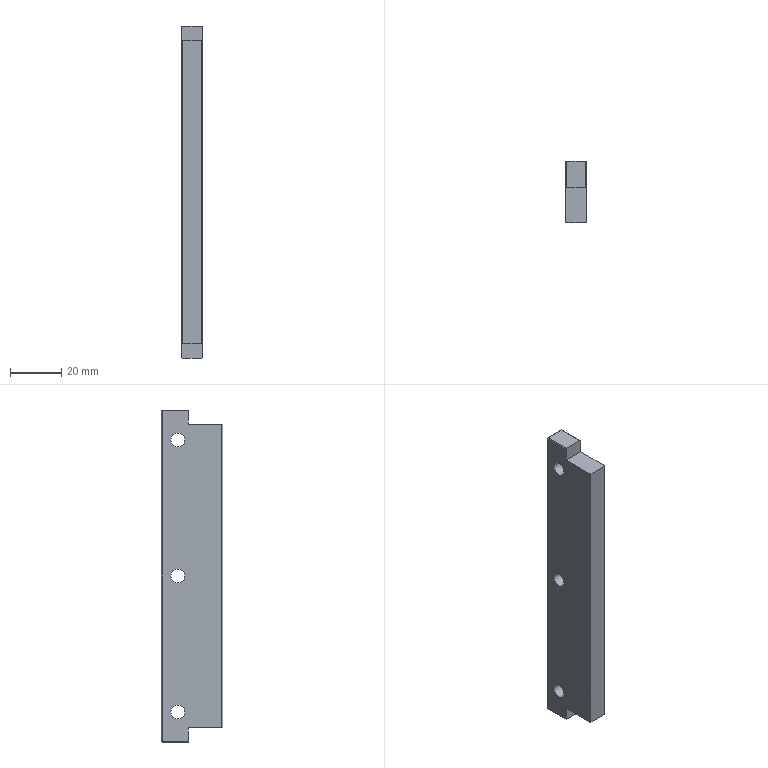Part | NX | 1 solid | 26 faces | box 8 x 24 x 130 mm | volume 23177 mm3 | plane 20 | cylinder 6 | commonest cylinder face diameters 5.5 x6
STEP:
#1=CARTESIAN_POINT('',(1727.3,110.5,87.2));
#2=VERTEX_POINT('',#1);
#3=CARTESIAN_POINT('',(1734.7,110.5,87.2));
#4=VERTEX_POINT('',#3);
#5=CARTESIAN_POINT('',(1731.,110.5,87.2));
#6=DIRECTION('',(1.,0.,0.));
#7=VECTOR('',#6,1000.);
#8=LINE('',#5,#7);
#9=EDGE_CURVE('',#2,#4,#8,.T.);
#10=ORIENTED_EDGE('',*,*,#9,.T.);
#11=CARTESIAN_POINT('',(1734.7,110.5,-42.2));
#12=VERTEX_POINT('',#11);
#13=CARTESIAN_POINT('',(1734.7,110.5,22.5));
#14=DIRECTION('',(0.,0.,1.));
#15=VECTOR('',#14,1000.);
#16=LINE('',#13,#15);
#17=EDGE_CURVE('',#12,#4,#16,.T.);
#18=ORIENTED_EDGE('',*,*,#17,.F.);
#19=CARTESIAN_POINT('',(1727.3,110.5,-42.2));
#20=VERTEX_POINT('',#19);
#21=CARTESIAN_POINT('',(1731.,110.5,-42.2));
#22=DIRECTION('',(-1.,0.,0.));
#23=VECTOR('',#22,1000.);
#24=LINE('',#21,#23);
#25=EDGE_CURVE('',#12,#20,#24,.T.);
#26=ORIENTED_EDGE('',*,*,#25,.T.);
#27=CARTESIAN_POINT('',(1727.3,110.5,22.5));
#28=DIRECTION('',(0.,0.,1.));
#29=VECTOR('',#28,1000.);
#30=LINE('',#27,#29);
#31=EDGE_CURVE('',#20,#2,#30,.T.);
#32=ORIENTED_EDGE('',*,*,#31,.T.);
#33=EDGE_LOOP('',(#10,#18,#26,#32));
#34=FACE_BOUND('',#33,.T.);
#35=CARTESIAN_POINT('',(1727.,110.5,93.5));
#36=DIRECTION('',(0.,1.,0.));
#37=DIRECTION('',(1.,0.,0.));
#38=AXIS2_PLACEMENT_3D('',#35,#36,#37);
#39=PLANE('',#38);
#40=ADVANCED_FACE('',(#34),#39,.T.);
#41=CARTESIAN_POINT('',(1734.7,100.,87.5));
#42=VERTEX_POINT('',#41);
#43=CARTESIAN_POINT('',(1727.3,100.,87.5));
#44=VERTEX_POINT('',#43);
#45=CARTESIAN_POINT('',(1727.,100.,87.5));
#46=DIRECTION('',(-1.,0.,0.));
#47=VECTOR('',#46,1000.);
#48=LINE('',#45,#47);
#49=EDGE_CURVE('',#42,#44,#48,.T.);
#50=ORIENTED_EDGE('',*,*,#49,.F.);
#51=CARTESIAN_POINT('',(1734.7,110.2,87.5));
#52=VERTEX_POINT('',#51);
#53=CARTESIAN_POINT('',(1734.7,103.803,87.5));
#54=DIRECTION('',(0.,-1.,0.));
#55=VECTOR('',#54,1000.);
#56=LINE('',#53,#55);
#57=EDGE_CURVE('',#52,#42,#56,.T.);
#58=ORIENTED_EDGE('',*,*,#57,.F.);
#59=CARTESIAN_POINT('',(1727.3,110.2,87.5));
#60=VERTEX_POINT('',#59);
#61=CARTESIAN_POINT('',(1731.,110.2,87.5));
#62=DIRECTION('',(1.,0.,0.));
#63=VECTOR('',#62,1000.);
#64=LINE('',#61,#63);
#65=EDGE_CURVE('',#60,#52,#64,.T.);
#66=ORIENTED_EDGE('',*,*,#65,.F.);
#67=CARTESIAN_POINT('',(1727.3,103.803,87.5));
#68=DIRECTION('',(0.,-1.,0.));
#69=VECTOR('',#68,1000.);
#70=LINE('',#67,#69);
#71=EDGE_CURVE('',#60,#44,#70,.T.);
#72=ORIENTED_EDGE('',*,*,#71,.T.);
#73=EDGE_LOOP('',(#50,#58,#66,#72));
#74=FACE_BOUND('',#73,.T.);
#75=CARTESIAN_POINT('',(1727.,88.5,87.5));
#76=DIRECTION('',(0.,0.,1.));
#77=DIRECTION('',(1.,0.,0.));
#78=AXIS2_PLACEMENT_3D('',#75,#76,#77);
#79=PLANE('',#78);
#80=ADVANCED_FACE('',(#74),#79,.T.);
#81=CARTESIAN_POINT('',(1727.,86.8,-37.));
#82=VERTEX_POINT('',#81);
#83=CARTESIAN_POINT('',(1727.,100.,-37.));
#84=VERTEX_POINT('',#83);
#85=CARTESIAN_POINT('',(1727.,0.,-37.));
#86=DIRECTION('',(0.,1.,0.));
#87=VECTOR('',#86,1000.);
#88=LINE('',#85,#87);
#89=EDGE_CURVE('',#82,#84,#88,.T.);
#90=ORIENTED_EDGE('',*,*,#89,.T.);
#91=CARTESIAN_POINT('',(1735.,100.,-37.));
#92=VERTEX_POINT('',#91);
#93=CARTESIAN_POINT('',(1727.,100.,-37.));
#94=DIRECTION('',(-1.,0.,0.));
#95=VECTOR('',#94,1000.);
#96=LINE('',#93,#95);
#97=EDGE_CURVE('',#92,#84,#96,.T.);
#98=ORIENTED_EDGE('',*,*,#97,.F.);
#99=CARTESIAN_POINT('',(1735.,86.8,-37.));
#100=VERTEX_POINT('',#99);
#101=CARTESIAN_POINT('',(1735.,103.803,-37.));
#102=DIRECTION('',(0.,-1.,0.));
#103=VECTOR('',#102,1000.);
#104=LINE('',#101,#103);
#105=EDGE_CURVE('',#92,#100,#104,.T.);
#106=ORIENTED_EDGE('',*,*,#105,.T.);
#107=CARTESIAN_POINT('',(1734.7,86.5,-37.));
#108=VERTEX_POINT('',#107);
#109=CARTESIAN_POINT('',(1752.003,103.803,-37.));
#110=DIRECTION('',(-0.7071,-0.7071,0.));
#111=VECTOR('',#110,1000.);
#112=LINE('',#109,#111);
#113=EDGE_CURVE('',#100,#108,#112,.T.);
#114=ORIENTED_EDGE('',*,*,#113,.T.);
#115=CARTESIAN_POINT('',(1727.3,86.5,-37.));
#116=VERTEX_POINT('',#115);
#117=CARTESIAN_POINT('',(1727.,86.5,-37.));
#118=DIRECTION('',(-1.,0.,0.));
#119=VECTOR('',#118,1000.);
#120=LINE('',#117,#119);
#121=EDGE_CURVE('',#108,#116,#120,.T.);
#122=ORIENTED_EDGE('',*,*,#121,.T.);
#123=CARTESIAN_POINT('',(1709.997,103.803,-37.));
#124=DIRECTION('',(0.7071,-0.7071,0.));
#125=VECTOR('',#124,1000.);
#126=LINE('',#123,#125);
#127=EDGE_CURVE('',#82,#116,#126,.T.);
#128=ORIENTED_EDGE('',*,*,#127,.F.);
#129=EDGE_LOOP('',(#90,#98,#106,#114,#122,#128));
#130=FACE_BOUND('',#129,.T.);
#131=CARTESIAN_POINT('',(1735.8,99.5,-37.));
#132=DIRECTION('',(0.,0.,1.));
#133=DIRECTION('',(1.,0.,0.));
#134=AXIS2_PLACEMENT_3D('',#131,#132,#133);
#135=PLANE('',#134);
#136=ADVANCED_FACE('',(#130),#135,.F.);
#137=CARTESIAN_POINT('',(1727.3,100.,-42.5));
#138=VERTEX_POINT('',#137);
#139=CARTESIAN_POINT('',(1727.3,110.2,-42.5));
#140=VERTEX_POINT('',#139);
#141=CARTESIAN_POINT('',(1727.3,103.803,-42.5));
#142=DIRECTION('',(0.,1.,0.));
#143=VECTOR('',#142,1000.);
#144=LINE('',#141,#143);
#145=EDGE_CURVE('',#138,#140,#144,.T.);
#146=ORIENTED_EDGE('',*,*,#145,.T.);
#147=CARTESIAN_POINT('',(1734.7,110.2,-42.5));
#148=VERTEX_POINT('',#147);
#149=CARTESIAN_POINT('',(1731.,110.2,-42.5));
#150=DIRECTION('',(-1.,0.,0.));
#151=VECTOR('',#150,1000.);
#152=LINE('',#149,#151);
#153=EDGE_CURVE('',#148,#140,#152,.T.);
#154=ORIENTED_EDGE('',*,*,#153,.F.);
#155=CARTESIAN_POINT('',(1734.7,100.,-42.5));
#156=VERTEX_POINT('',#155);
#157=CARTESIAN_POINT('',(1734.7,103.803,-42.5));
#158=DIRECTION('',(0.,1.,0.));
#159=VECTOR('',#158,1000.);
#160=LINE('',#157,#159);
#161=EDGE_CURVE('',#156,#148,#160,.T.);
#162=ORIENTED_EDGE('',*,*,#161,.F.);
#163=CARTESIAN_POINT('',(1727.,100.,-42.5));
#164=DIRECTION('',(1.,0.,0.));
#165=VECTOR('',#164,1000.);
#166=LINE('',#163,#165);
#167=EDGE_CURVE('',#138,#156,#166,.T.);
#168=ORIENTED_EDGE('',*,*,#167,.F.);
#169=EDGE_LOOP('',(#146,#154,#162,#168));
#170=FACE_BOUND('',#169,.T.);
#171=CARTESIAN_POINT('',(1727.,110.5,-42.5));
#172=DIRECTION('',(0.,0.,-1.));
#173=DIRECTION('',(0.,-1.,0.));
#174=AXIS2_PLACEMENT_3D('',#171,#172,#173);
#175=PLANE('',#174);
#176=ADVANCED_FACE('',(#170),#175,.T.);
#177=ORIENTED_EDGE('',*,*,#121,.F.);
#178=CARTESIAN_POINT('',(1734.7,86.5,82.));
#179=VERTEX_POINT('',#178);
#180=CARTESIAN_POINT('',(1734.7,86.5,-14.233));
#181=DIRECTION('',(0.,0.,-1.));
#182=VECTOR('',#181,1000.);
#183=LINE('',#180,#182);
#184=EDGE_CURVE('',#179,#108,#183,.T.);
#185=ORIENTED_EDGE('',*,*,#184,.F.);
#186=CARTESIAN_POINT('',(1727.3,86.5,82.));
#187=VERTEX_POINT('',#186);
#188=CARTESIAN_POINT('',(1727.,86.5,82.));
#189=DIRECTION('',(1.,0.,0.));
#190=VECTOR('',#189,1000.);
#191=LINE('',#188,#190);
#192=EDGE_CURVE('',#187,#179,#191,.T.);
#193=ORIENTED_EDGE('',*,*,#192,.F.);
#194=CARTESIAN_POINT('',(1727.3,86.5,-14.233));
#195=DIRECTION('',(0.,0.,-1.));
#196=VECTOR('',#195,1000.);
#197=LINE('',#194,#196);
#198=EDGE_CURVE('',#187,#116,#197,.T.);
#199=ORIENTED_EDGE('',*,*,#198,.T.);
#200=EDGE_LOOP('',(#177,#185,#193,#199));
#201=FACE_BOUND('',#200,.T.);
#202=CARTESIAN_POINT('',(1727.,86.5,-48.5));
#203=DIRECTION('',(0.,-1.,0.));
#204=DIRECTION('',(0.,0.,-1.));
#205=AXIS2_PLACEMENT_3D('',#202,#203,#204);
#206=PLANE('',#205);
#207=ADVANCED_FACE('',(#201),#206,.T.);
#208=ORIENTED_EDGE('',*,*,#25,.F.);
#209=CARTESIAN_POINT('',(1734.85,110.35,-42.35));
#210=VERTEX_POINT('',#209);
#211=CARTESIAN_POINT('',(1706.733,138.467,-14.233));
#212=DIRECTION('',(0.5774,-0.5774,-0.5774));
#213=VECTOR('',#212,1000.);
#214=LINE('',#211,#213);
#215=EDGE_CURVE('',#12,#210,#214,.T.);
#216=ORIENTED_EDGE('',*,*,#215,.T.);
#217=CARTESIAN_POINT('',(1762.967,138.467,-14.233));
#218=DIRECTION('',(0.5774,0.5774,0.5774));
#219=VECTOR('',#218,1000.);
#220=LINE('',#217,#219);
#221=EDGE_CURVE('',#148,#210,#220,.T.);
#222=ORIENTED_EDGE('',*,*,#221,.F.);
#223=ORIENTED_EDGE('',*,*,#153,.T.);
#224=CARTESIAN_POINT('',(1727.15,110.35,-42.35));
#225=VERTEX_POINT('',#224);
#226=CARTESIAN_POINT('',(1699.033,138.467,-14.233));
#227=DIRECTION('',(-0.5774,0.5774,0.5774));
#228=VECTOR('',#227,1000.);
#229=LINE('',#226,#228);
#230=EDGE_CURVE('',#140,#225,#229,.T.);
#231=ORIENTED_EDGE('',*,*,#230,.T.);
#232=CARTESIAN_POINT('',(1755.267,138.467,-14.233));
#233=DIRECTION('',(-0.5774,-0.5774,-0.5774));
#234=VECTOR('',#233,1000.);
#235=LINE('',#232,#234);
#236=EDGE_CURVE('',#20,#225,#235,.T.);
#237=ORIENTED_EDGE('',*,*,#236,.F.);
#238=EDGE_LOOP('',(#208,#216,#222,#223,#231,#237));
#239=FACE_BOUND('',#238,.T.);
#240=CARTESIAN_POINT('',(1731.,110.35,-42.35));
#241=DIRECTION('',(0.,0.7071,-0.7071));
#242=DIRECTION('',(-1.,0.,0.));
#243=AXIS2_PLACEMENT_3D('',#240,#241,#242);
#244=PLANE('',#243);
#245=ADVANCED_FACE('',(#239),#244,.T.);
#246=ORIENTED_EDGE('',*,*,#9,.F.);
#247=CARTESIAN_POINT('',(1727.15,110.35,87.35));
#248=VERTEX_POINT('',#247);
#249=CARTESIAN_POINT('',(1727.,110.2,87.5));
#250=DIRECTION('',(-0.5774,-0.5774,0.5774));
#251=VECTOR('',#250,1000.);
#252=LINE('',#249,#251);
#253=EDGE_CURVE('',#2,#248,#252,.T.);
#254=ORIENTED_EDGE('',*,*,#253,.T.);
#255=CARTESIAN_POINT('',(1733.697,103.803,93.897));
#256=DIRECTION('',(-0.5774,0.5774,-0.5774));
#257=VECTOR('',#256,1000.);
#258=LINE('',#255,#257);
#259=EDGE_CURVE('',#60,#248,#258,.T.);
#260=ORIENTED_EDGE('',*,*,#259,.F.);
#261=ORIENTED_EDGE('',*,*,#65,.T.);
#262=CARTESIAN_POINT('',(1734.85,110.35,87.35));
#263=VERTEX_POINT('',#262);
#264=CARTESIAN_POINT('',(1728.303,103.803,93.897));
#265=DIRECTION('',(0.5774,0.5774,-0.5774));
#266=VECTOR('',#265,1000.);
#267=LINE('',#264,#266);
#268=EDGE_CURVE('',#52,#263,#267,.T.);
#269=ORIENTED_EDGE('',*,*,#268,.T.);
#270=CARTESIAN_POINT('',(1741.397,103.803,93.897));
#271=DIRECTION('',(0.5774,-0.5774,0.5774));
#272=VECTOR('',#271,1000.);
#273=LINE('',#270,#272);
#274=EDGE_CURVE('',#4,#263,#273,.T.);
#275=ORIENTED_EDGE('',*,*,#274,.F.);
#276=EDGE_LOOP('',(#246,#254,#260,#261,#269,#275));
#277=FACE_BOUND('',#276,.T.);
#278=CARTESIAN_POINT('',(1731.,110.35,87.35));
#279=DIRECTION('',(0.,0.7071,0.7071));
#280=DIRECTION('',(1.,0.,0.));
#281=AXIS2_PLACEMENT_3D('',#278,#279,#280);
#282=PLANE('',#281);
#283=ADVANCED_FACE('',(#277),#282,.T.);
#284=CARTESIAN_POINT('',(1727.,100.,-42.2));
#285=VERTEX_POINT('',#284);
#286=CARTESIAN_POINT('',(1727.,100.,0.));
#287=DIRECTION('',(0.,0.,-1.));
#288=VECTOR('',#287,1000.);
#289=LINE('',#286,#288);
#290=EDGE_CURVE('',#84,#285,#289,.T.);
#291=ORIENTED_EDGE('',*,*,#290,.T.);
#292=CARTESIAN_POINT('',(1699.033,100.,-14.233));
#293=DIRECTION('',(-0.7071,0.,0.7071));
#294=VECTOR('',#293,1000.);
#295=LINE('',#292,#294);
#296=EDGE_CURVE('',#138,#285,#295,.T.);
#297=ORIENTED_EDGE('',*,*,#296,.F.);
#298=ORIENTED_EDGE('',*,*,#167,.T.);
#299=CARTESIAN_POINT('',(1735.,100.,-42.2));
#300=VERTEX_POINT('',#299);
#301=CARTESIAN_POINT('',(1762.967,100.,-14.233));
#302=DIRECTION('',(0.7071,0.,0.7071));
#303=VECTOR('',#302,1000.);
#304=LINE('',#301,#303);
#305=EDGE_CURVE('',#156,#300,#304,.T.);
#306=ORIENTED_EDGE('',*,*,#305,.T.);
#307=CARTESIAN_POINT('',(1735.,100.,-14.233));
#308=DIRECTION('',(0.,0.,1.));
#309=VECTOR('',#308,1000.);
#310=LINE('',#307,#309);
#311=EDGE_CURVE('',#300,#92,#310,.T.);
#312=ORIENTED_EDGE('',*,*,#311,.T.);
#313=ORIENTED_EDGE('',*,*,#97,.T.);
#314=EDGE_LOOP('',(#291,#297,#298,#306,#312,#313));
#315=FACE_BOUND('',#314,.T.);
#316=CARTESIAN_POINT('',(1735.8,100.,-79.5));
#317=DIRECTION('',(0.,1.,0.));
#318=DIRECTION('',(1.,0.,0.));
#319=AXIS2_PLACEMENT_3D('',#316,#317,#318);
#320=PLANE('',#319);
#321=ADVANCED_FACE('',(#315),#320,.F.);
#322=CARTESIAN_POINT('',(1735.,86.8,82.));
#323=VERTEX_POINT('',#322);
#324=CARTESIAN_POINT('',(1735.,100.,82.));
#325=VERTEX_POINT('',#324);
#326=CARTESIAN_POINT('',(1735.,103.803,82.));
#327=DIRECTION('',(0.,1.,0.));
#328=VECTOR('',#327,1000.);
#329=LINE('',#326,#328);
#330=EDGE_CURVE('',#323,#325,#329,.T.);
#331=ORIENTED_EDGE('',*,*,#330,.F.);
#332=CARTESIAN_POINT('',(1735.,86.8,-14.233));
#333=DIRECTION('',(0.,0.,-1.));
#334=VECTOR('',#333,1000.);
#335=LINE('',#332,#334);
#336=EDGE_CURVE('',#323,#100,#335,.T.);
#337=ORIENTED_EDGE('',*,*,#336,.T.);
#338=ORIENTED_EDGE('',*,*,#105,.F.);
#339=ORIENTED_EDGE('',*,*,#311,.F.);
#340=CARTESIAN_POINT('',(1735.,110.2,-42.2));
#341=VERTEX_POINT('',#340);
#342=CARTESIAN_POINT('',(1735.,103.803,-42.2));
#343=DIRECTION('',(0.,1.,0.));
#344=VECTOR('',#343,1000.);
#345=LINE('',#342,#344);
#346=EDGE_CURVE('',#300,#341,#345,.T.);
#347=ORIENTED_EDGE('',*,*,#346,.T.);
#348=CARTESIAN_POINT('',(1735.,110.2,87.2));
#349=VERTEX_POINT('',#348);
#350=CARTESIAN_POINT('',(1735.,110.2,22.5));
#351=DIRECTION('',(0.,0.,1.));
#352=VECTOR('',#351,1000.);
#353=LINE('',#350,#352);
#354=EDGE_CURVE('',#341,#349,#353,.T.);
#355=ORIENTED_EDGE('',*,*,#354,.T.);
#356=CARTESIAN_POINT('',(1735.,100.,87.2));
#357=VERTEX_POINT('',#356);
#358=CARTESIAN_POINT('',(1735.,103.803,87.2));
#359=DIRECTION('',(0.,-1.,0.));
#360=VECTOR('',#359,1000.);
#361=LINE('',#358,#360);
#362=EDGE_CURVE('',#349,#357,#361,.T.);
#363=ORIENTED_EDGE('',*,*,#362,.T.);
#364=CARTESIAN_POINT('',(1735.,100.,-14.233));
#365=DIRECTION('',(0.,0.,1.));
#366=VECTOR('',#365,1000.);
#367=LINE('',#364,#366);
#368=EDGE_CURVE('',#325,#357,#367,.T.);
#369=ORIENTED_EDGE('',*,*,#368,.F.);
#370=EDGE_LOOP('',(#331,#337,#338,#339,#347,#355,#363,#369));
#371=FACE_BOUND('',#370,.T.);
#372=CARTESIAN_POINT('',(1735.,101.25,75.75));
#373=VERTEX_POINT('',#372);
#374=CARTESIAN_POINT('',(1735.,106.75,75.75));
#375=VERTEX_POINT('',#374);
#376=CARTESIAN_POINT('',(1735.,104.,75.75));
#377=DIRECTION('',(1.,0.,0.));
#378=DIRECTION('',(0.,1.,0.));
#379=AXIS2_PLACEMENT_3D('',#376,#377,#378);
#380=CIRCLE('',#379,2.75);
#381=EDGE_CURVE('',#373,#375,#380,.T.);
#382=ORIENTED_EDGE('',*,*,#381,.F.);
#383=CARTESIAN_POINT('',(1735.,104.,75.75));
#384=DIRECTION('',(1.,0.,0.));
#385=DIRECTION('',(0.,1.,0.));
#386=AXIS2_PLACEMENT_3D('',#383,#384,#385);
#387=CIRCLE('',#386,2.75);
#388=EDGE_CURVE('',#375,#373,#387,.T.);
#389=ORIENTED_EDGE('',*,*,#388,.F.);
#390=EDGE_LOOP('',(#382,#389));
#391=FACE_BOUND('',#390,.T.);
#392=CARTESIAN_POINT('',(1735.,101.25,-30.75));
#393=VERTEX_POINT('',#392);
#394=CARTESIAN_POINT('',(1735.,106.75,-30.75));
#395=VERTEX_POINT('',#394);
#396=CARTESIAN_POINT('',(1735.,104.,-30.75));
#397=DIRECTION('',(1.,0.,0.));
#398=DIRECTION('',(0.,1.,0.));
#399=AXIS2_PLACEMENT_3D('',#396,#397,#398);
#400=CIRCLE('',#399,2.75);
#401=EDGE_CURVE('',#393,#395,#400,.T.);
#402=ORIENTED_EDGE('',*,*,#401,.F.);
#403=CARTESIAN_POINT('',(1735.,104.,-30.75));
#404=DIRECTION('',(1.,0.,0.));
#405=DIRECTION('',(0.,1.,0.));
#406=AXIS2_PLACEMENT_3D('',#403,#404,#405);
#407=CIRCLE('',#406,2.75);
#408=EDGE_CURVE('',#395,#393,#407,.T.);
#409=ORIENTED_EDGE('',*,*,#408,.F.);
#410=EDGE_LOOP('',(#402,#409));
#411=FACE_BOUND('',#410,.T.);
#412=CARTESIAN_POINT('',(1735.,101.25,22.5));
#413=VERTEX_POINT('',#412);
#414=CARTESIAN_POINT('',(1735.,106.75,22.5));
#415=VERTEX_POINT('',#414);
#416=CARTESIAN_POINT('',(1735.,104.,22.5));
#417=DIRECTION('',(1.,0.,0.));
#418=DIRECTION('',(0.,1.,0.));
#419=AXIS2_PLACEMENT_3D('',#416,#417,#418);
#420=CIRCLE('',#419,2.75);
#421=EDGE_CURVE('',#413,#415,#420,.T.);
#422=ORIENTED_EDGE('',*,*,#421,.F.);
#423=CARTESIAN_POINT('',(1735.,104.,22.5));
#424=DIRECTION('',(1.,0.,0.));
#425=DIRECTION('',(0.,1.,0.));
#426=AXIS2_PLACEMENT_3D('',#423,#424,#425);
#427=CIRCLE('',#426,2.75);
#428=EDGE_CURVE('',#415,#413,#427,.T.);
#429=ORIENTED_EDGE('',*,*,#428,.F.);
#430=EDGE_LOOP('',(#422,#429));
#431=FACE_BOUND('',#430,.T.);
#432=CARTESIAN_POINT('',(1735.,103.803,-14.233));
#433=DIRECTION('',(1.,0.,0.));
#434=DIRECTION('',(0.,1.,0.));
#435=AXIS2_PLACEMENT_3D('',#432,#433,#434);
#436=PLANE('',#435);
#437=ADVANCED_FACE('',(#371,#391,#411,#431),#436,.T.);
#438=CARTESIAN_POINT('',(1727.,101.25,75.75));
#439=VERTEX_POINT('',#438);
#440=CARTESIAN_POINT('',(1727.,106.75,75.75));
#441=VERTEX_POINT('',#440);
#442=CARTESIAN_POINT('',(1727.,104.,75.75));
#443=DIRECTION('',(1.,0.,0.));
#444=DIRECTION('',(0.,1.,0.));
#445=AXIS2_PLACEMENT_3D('',#442,#443,#444);
#446=CIRCLE('',#445,2.75);
#447=EDGE_CURVE('',#439,#441,#446,.T.);
#448=ORIENTED_EDGE('',*,*,#447,.F.);
#449=CARTESIAN_POINT('',(1735.,101.25,75.75));
#450=DIRECTION('',(1.,0.,0.));
#451=VECTOR('',#450,1000.);
#452=LINE('',#449,#451);
#453=EDGE_CURVE('',#439,#373,#452,.T.);
#454=ORIENTED_EDGE('',*,*,#453,.T.);
#455=ORIENTED_EDGE('',*,*,#381,.T.);
#456=CARTESIAN_POINT('',(1735.,106.75,75.75));
#457=DIRECTION('',(1.,0.,0.));
#458=VECTOR('',#457,1000.);
#459=LINE('',#456,#458);
#460=EDGE_CURVE('',#441,#375,#459,.T.);
#461=ORIENTED_EDGE('',*,*,#460,.F.);
#462=EDGE_LOOP('',(#448,#454,#455,#461));
#463=FACE_BOUND('',#462,.T.);
#464=CARTESIAN_POINT('',(1735.,104.,75.75));
#465=DIRECTION('',(1.,0.,0.));
#466=DIRECTION('',(0.,1.,0.));
#467=AXIS2_PLACEMENT_3D('',#464,#465,#466);
#468=CYLINDRICAL_SURFACE('',#467,2.75);
#469=ADVANCED_FACE('',(#463),#468,.F.);
#470=CARTESIAN_POINT('',(1727.,100.,82.));
#471=VERTEX_POINT('',#470);
#472=CARTESIAN_POINT('',(1727.,86.8,82.));
#473=VERTEX_POINT('',#472);
#474=CARTESIAN_POINT('',(1727.,0.,82.));
#475=DIRECTION('',(0.,-1.,0.));
#476=VECTOR('',#475,1000.);
#477=LINE('',#474,#476);
#478=EDGE_CURVE('',#471,#473,#477,.T.);
#479=ORIENTED_EDGE('',*,*,#478,.T.);
#480=CARTESIAN_POINT('',(1709.997,103.803,82.));
#481=DIRECTION('',(-0.7071,0.7071,0.));
#482=VECTOR('',#481,1000.);
#483=LINE('',#480,#482);
#484=EDGE_CURVE('',#187,#473,#483,.T.);
#485=ORIENTED_EDGE('',*,*,#484,.F.);
#486=ORIENTED_EDGE('',*,*,#192,.T.);
#487=CARTESIAN_POINT('',(1752.003,103.803,82.));
#488=DIRECTION('',(0.7071,0.7071,0.));
#489=VECTOR('',#488,1000.);
#490=LINE('',#487,#489);
#491=EDGE_CURVE('',#179,#323,#490,.T.);
#492=ORIENTED_EDGE('',*,*,#491,.T.);
#493=ORIENTED_EDGE('',*,*,#330,.T.);
#494=CARTESIAN_POINT('',(1727.,100.,82.));
#495=DIRECTION('',(1.,0.,0.));
#496=VECTOR('',#495,1000.);
#497=LINE('',#494,#496);
#498=EDGE_CURVE('',#471,#325,#497,.T.);
#499=ORIENTED_EDGE('',*,*,#498,.F.);
#500=EDGE_LOOP('',(#479,#485,#486,#492,#493,#499));
#501=FACE_BOUND('',#500,.T.);
#502=CARTESIAN_POINT('',(1735.8,54.5,82.));
#503=DIRECTION('',(0.,0.,-1.));
#504=DIRECTION('',(0.,-1.,0.));
#505=AXIS2_PLACEMENT_3D('',#502,#503,#504);
#506=PLANE('',#505);
#507=ADVANCED_FACE('',(#501),#506,.F.);
#508=CARTESIAN_POINT('',(1727.,101.25,22.5));
#509=VERTEX_POINT('',#508);
#510=CARTESIAN_POINT('',(1727.,106.75,22.5));
#511=VERTEX_POINT('',#510);
#512=CARTESIAN_POINT('',(1727.,104.,22.5));
#513=DIRECTION('',(1.,0.,0.));
#514=DIRECTION('',(0.,1.,0.));
#515=AXIS2_PLACEMENT_3D('',#512,#513,#514);
#516=CIRCLE('',#515,2.75);
#517=EDGE_CURVE('',#509,#511,#516,.T.);
#518=ORIENTED_EDGE('',*,*,#517,.F.);
#519=CARTESIAN_POINT('',(1735.,101.25,22.5));
#520=DIRECTION('',(1.,0.,0.));
#521=VECTOR('',#520,1000.);
#522=LINE('',#519,#521);
#523=EDGE_CURVE('',#509,#413,#522,.T.);
#524=ORIENTED_EDGE('',*,*,#523,.T.);
#525=ORIENTED_EDGE('',*,*,#421,.T.);
#526=CARTESIAN_POINT('',(1735.,106.75,22.5));
#527=DIRECTION('',(1.,0.,0.));
#528=VECTOR('',#527,1000.);
#529=LINE('',#526,#528);
#530=EDGE_CURVE('',#511,#415,#529,.T.);
#531=ORIENTED_EDGE('',*,*,#530,.F.);
#532=EDGE_LOOP('',(#518,#524,#525,#531));
#533=FACE_BOUND('',#532,.T.);
#534=CARTESIAN_POINT('',(1735.,104.,22.5));
#535=DIRECTION('',(1.,0.,0.));
#536=DIRECTION('',(0.,1.,0.));
#537=AXIS2_PLACEMENT_3D('',#534,#535,#536);
#538=CYLINDRICAL_SURFACE('',#537,2.75);
#539=ADVANCED_FACE('',(#533),#538,.F.);
#540=CARTESIAN_POINT('',(1727.,100.,87.2));
#541=VERTEX_POINT('',#540);
#542=CARTESIAN_POINT('',(1727.,100.,87.2));
#543=DIRECTION('',(0.7071,0.,0.7071));
#544=VECTOR('',#543,1000.);
#545=LINE('',#542,#544);
#546=EDGE_CURVE('',#541,#44,#545,.T.);
#547=ORIENTED_EDGE('',*,*,#546,.T.);
#548=ORIENTED_EDGE('',*,*,#71,.F.);
#549=ORIENTED_EDGE('',*,*,#259,.T.);
#550=CARTESIAN_POINT('',(1727.,110.2,87.2));
#551=VERTEX_POINT('',#550);
#552=CARTESIAN_POINT('',(1727.,110.2,87.2));
#553=DIRECTION('',(0.5774,0.5774,0.5774));
#554=VECTOR('',#553,1000.);
#555=LINE('',#552,#554);
#556=EDGE_CURVE('',#551,#248,#555,.T.);
#557=ORIENTED_EDGE('',*,*,#556,.F.);
#558=CARTESIAN_POINT('',(1727.,0.,87.2));
#559=DIRECTION('',(0.,-1.,0.));
#560=VECTOR('',#559,1000.);
#561=LINE('',#558,#560);
#562=EDGE_CURVE('',#551,#541,#561,.T.);
#563=ORIENTED_EDGE('',*,*,#562,.T.);
#564=EDGE_LOOP('',(#547,#548,#549,#557,#563));
#565=FACE_BOUND('',#564,.T.);
#566=CARTESIAN_POINT('',(1727.15,98.5,87.35));
#567=DIRECTION('',(0.7071,0.,-0.7071));
#568=DIRECTION('',(0.,-1.,0.));
#569=AXIS2_PLACEMENT_3D('',#566,#567,#568);
#570=PLANE('',#569);
#571=ADVANCED_FACE('',(#565),#570,.F.);
#572=ORIENTED_EDGE('',*,*,#401,.T.);
#573=CARTESIAN_POINT('',(1727.,106.75,-30.75));
#574=VERTEX_POINT('',#573);
#575=CARTESIAN_POINT('',(1735.,106.75,-30.75));
#576=DIRECTION('',(1.,0.,0.));
#577=VECTOR('',#576,1000.);
#578=LINE('',#575,#577);
#579=EDGE_CURVE('',#574,#395,#578,.T.);
#580=ORIENTED_EDGE('',*,*,#579,.F.);
#581=CARTESIAN_POINT('',(1727.,101.25,-30.75));
#582=VERTEX_POINT('',#581);
#583=CARTESIAN_POINT('',(1727.,104.,-30.75));
#584=DIRECTION('',(1.,0.,0.));
#585=DIRECTION('',(0.,1.,0.));
#586=AXIS2_PLACEMENT_3D('',#583,#584,#585);
#587=CIRCLE('',#586,2.75);
#588=EDGE_CURVE('',#582,#574,#587,.T.);
#589=ORIENTED_EDGE('',*,*,#588,.F.);
#590=CARTESIAN_POINT('',(1735.,101.25,-30.75));
#591=DIRECTION('',(1.,0.,0.));
#592=VECTOR('',#591,1000.);
#593=LINE('',#590,#592);
#594=EDGE_CURVE('',#582,#393,#593,.T.);
#595=ORIENTED_EDGE('',*,*,#594,.T.);
#596=EDGE_LOOP('',(#572,#580,#589,#595));
#597=FACE_BOUND('',#596,.T.);
#598=CARTESIAN_POINT('',(1735.,104.,-30.75));
#599=DIRECTION('',(1.,0.,0.));
#600=DIRECTION('',(0.,1.,0.));
#601=AXIS2_PLACEMENT_3D('',#598,#599,#600);
#602=CYLINDRICAL_SURFACE('',#601,2.75);
#603=ADVANCED_FACE('',(#597),#602,.F.);
#604=CARTESIAN_POINT('',(1727.,110.2,-42.2));
#605=VERTEX_POINT('',#604);
#606=CARTESIAN_POINT('',(1727.,0.,-42.2));
#607=DIRECTION('',(0.,1.,0.));
#608=VECTOR('',#607,1000.);
#609=LINE('',#606,#608);
#610=EDGE_CURVE('',#285,#605,#609,.T.);
#611=ORIENTED_EDGE('',*,*,#610,.T.);
#612=CARTESIAN_POINT('',(1699.033,82.233,-14.233));
#613=DIRECTION('',(0.5774,0.5774,-0.5774));
#614=VECTOR('',#613,1000.);
#615=LINE('',#612,#614);
#616=EDGE_CURVE('',#605,#225,#615,.T.);
#617=ORIENTED_EDGE('',*,*,#616,.T.);
#618=ORIENTED_EDGE('',*,*,#230,.F.);
#619=ORIENTED_EDGE('',*,*,#145,.F.);
#620=ORIENTED_EDGE('',*,*,#296,.T.);
#621=EDGE_LOOP('',(#611,#617,#618,#619,#620));
#622=FACE_BOUND('',#621,.T.);
#623=CARTESIAN_POINT('',(1727.15,98.5,-42.35));
#624=DIRECTION('',(0.7071,0.,0.7071));
#625=DIRECTION('',(0.,-1.,0.));
#626=AXIS2_PLACEMENT_3D('',#623,#624,#625);
#627=PLANE('',#626);
#628=ADVANCED_FACE('',(#622),#627,.F.);
#629=ORIENTED_EDGE('',*,*,#113,.F.);
#630=ORIENTED_EDGE('',*,*,#336,.F.);
#631=ORIENTED_EDGE('',*,*,#491,.F.);
#632=ORIENTED_EDGE('',*,*,#184,.T.);
#633=EDGE_LOOP('',(#629,#630,#631,#632));
#634=FACE_BOUND('',#633,.T.);
#635=CARTESIAN_POINT('',(1734.85,86.65,22.5));
#636=DIRECTION('',(0.7071,-0.7071,0.));
#637=DIRECTION('',(0.,0.,-1.));
#638=AXIS2_PLACEMENT_3D('',#635,#636,#637);
#639=PLANE('',#638);
#640=ADVANCED_FACE('',(#634),#639,.T.);
#641=ORIENTED_EDGE('',*,*,#346,.F.);
#642=ORIENTED_EDGE('',*,*,#305,.F.);
#643=ORIENTED_EDGE('',*,*,#161,.T.);
#644=ORIENTED_EDGE('',*,*,#221,.T.);
#645=CARTESIAN_POINT('',(1762.967,82.233,-14.233));
#646=DIRECTION('',(0.5774,-0.5774,0.5774));
#647=VECTOR('',#646,1000.);
#648=LINE('',#645,#647);
#649=EDGE_CURVE('',#210,#341,#648,.T.);
#650=ORIENTED_EDGE('',*,*,#649,.T.);
#651=EDGE_LOOP('',(#641,#642,#643,#644,#650));
#652=FACE_BOUND('',#651,.T.);
#653=CARTESIAN_POINT('',(1734.85,98.5,-42.35));
#654=DIRECTION('',(0.7071,0.,-0.7071));
#655=DIRECTION('',(0.,-1.,0.));
#656=AXIS2_PLACEMENT_3D('',#653,#654,#655);
#657=PLANE('',#656);
#658=ADVANCED_FACE('',(#652),#657,.T.);
#659=ORIENTED_EDGE('',*,*,#354,.F.);
#660=ORIENTED_EDGE('',*,*,#649,.F.);
#661=ORIENTED_EDGE('',*,*,#215,.F.);
#662=ORIENTED_EDGE('',*,*,#17,.T.);
#663=ORIENTED_EDGE('',*,*,#274,.T.);
#664=CARTESIAN_POINT('',(1727.,118.2,95.2));
#665=DIRECTION('',(0.5774,-0.5774,-0.5774));
#666=VECTOR('',#665,1000.);
#667=LINE('',#664,#666);
#668=EDGE_CURVE('',#263,#349,#667,.T.);
#669=ORIENTED_EDGE('',*,*,#668,.T.);
#670=EDGE_LOOP('',(#659,#660,#661,#662,#663,#669));
#671=FACE_BOUND('',#670,.T.);
#672=CARTESIAN_POINT('',(1734.85,110.35,22.5));
#673=DIRECTION('',(0.7071,0.7071,0.));
#674=DIRECTION('',(0.,0.,-1.));
#675=AXIS2_PLACEMENT_3D('',#672,#673,#674);
#676=PLANE('',#675);
#677=ADVANCED_FACE('',(#671),#676,.T.);
#678=CARTESIAN_POINT('',(1727.,100.,95.2));
#679=DIRECTION('',(-0.7071,0.,0.7071));
#680=VECTOR('',#679,1000.);
#681=LINE('',#678,#680);
#682=EDGE_CURVE('',#357,#42,#681,.T.);
#683=ORIENTED_EDGE('',*,*,#682,.F.);
#684=ORIENTED_EDGE('',*,*,#362,.F.);
#685=ORIENTED_EDGE('',*,*,#668,.F.);
#686=ORIENTED_EDGE('',*,*,#268,.F.);
#687=ORIENTED_EDGE('',*,*,#57,.T.);
#688=EDGE_LOOP('',(#683,#684,#685,#686,#687));
#689=FACE_BOUND('',#688,.T.);
#690=CARTESIAN_POINT('',(1734.85,98.5,87.35));
#691=DIRECTION('',(0.7071,0.,0.7071));
#692=DIRECTION('',(0.,-1.,0.));
#693=AXIS2_PLACEMENT_3D('',#690,#691,#692);
#694=PLANE('',#693);
#695=ADVANCED_FACE('',(#689),#694,.T.);
#696=ORIENTED_EDGE('',*,*,#478,.F.);
#697=CARTESIAN_POINT('',(1727.,100.,0.));
#698=DIRECTION('',(0.,0.,-1.));
#699=VECTOR('',#698,1000.);
#700=LINE('',#697,#699);
#701=EDGE_CURVE('',#541,#471,#700,.T.);
#702=ORIENTED_EDGE('',*,*,#701,.F.);
#703=ORIENTED_EDGE('',*,*,#562,.F.);
#704=CARTESIAN_POINT('',(1727.,110.2,0.));
#705=DIRECTION('',(0.,0.,1.));
#706=VECTOR('',#705,1000.);
#707=LINE('',#704,#706);
#708=EDGE_CURVE('',#605,#551,#707,.T.);
#709=ORIENTED_EDGE('',*,*,#708,.F.);
#710=ORIENTED_EDGE('',*,*,#610,.F.);
#711=ORIENTED_EDGE('',*,*,#290,.F.);
#712=ORIENTED_EDGE('',*,*,#89,.F.);
#713=CARTESIAN_POINT('',(1727.,86.8,0.));
#714=DIRECTION('',(0.,0.,-1.));
#715=VECTOR('',#714,1000.);
#716=LINE('',#713,#715);
#717=EDGE_CURVE('',#473,#82,#716,.T.);
#718=ORIENTED_EDGE('',*,*,#717,.F.);
#719=EDGE_LOOP('',(#696,#702,#703,#709,#710,#711,#712,#718));
#720=FACE_BOUND('',#719,.T.);
#721=ORIENTED_EDGE('',*,*,#588,.T.);
#722=CARTESIAN_POINT('',(1727.,104.,-30.75));
#723=DIRECTION('',(1.,0.,0.));
#724=DIRECTION('',(0.,1.,0.));
#725=AXIS2_PLACEMENT_3D('',#722,#723,#724);
#726=CIRCLE('',#725,2.75);
#727=EDGE_CURVE('',#574,#582,#726,.T.);
#728=ORIENTED_EDGE('',*,*,#727,.T.);
#729=EDGE_LOOP('',(#721,#728));
#730=FACE_BOUND('',#729,.T.);
#731=ORIENTED_EDGE('',*,*,#517,.T.);
#732=CARTESIAN_POINT('',(1727.,104.,22.5));
#733=DIRECTION('',(1.,0.,0.));
#734=DIRECTION('',(0.,1.,0.));
#735=AXIS2_PLACEMENT_3D('',#732,#733,#734);
#736=CIRCLE('',#735,2.75);
#737=EDGE_CURVE('',#511,#509,#736,.T.);
#738=ORIENTED_EDGE('',*,*,#737,.T.);
#739=EDGE_LOOP('',(#731,#738));
#740=FACE_BOUND('',#739,.T.);
#741=ORIENTED_EDGE('',*,*,#447,.T.);
#742=CARTESIAN_POINT('',(1727.,104.,75.75));
#743=DIRECTION('',(1.,0.,0.));
#744=DIRECTION('',(0.,1.,0.));
#745=AXIS2_PLACEMENT_3D('',#742,#743,#744);
#746=CIRCLE('',#745,2.75);
#747=EDGE_CURVE('',#441,#439,#746,.T.);
#748=ORIENTED_EDGE('',*,*,#747,.T.);
#749=EDGE_LOOP('',(#741,#748));
#750=FACE_BOUND('',#749,.T.);
#751=CARTESIAN_POINT('',(1727.,103.803,-14.233));
#752=DIRECTION('',(1.,0.,0.));
#753=DIRECTION('',(0.,1.,0.));
#754=AXIS2_PLACEMENT_3D('',#751,#752,#753);
#755=PLANE('',#754);
#756=ADVANCED_FACE('',(#720,#730,#740,#750),#755,.F.);
#757=ORIENTED_EDGE('',*,*,#127,.T.);
#758=ORIENTED_EDGE('',*,*,#198,.F.);
#759=ORIENTED_EDGE('',*,*,#484,.T.);
#760=ORIENTED_EDGE('',*,*,#717,.T.);
#761=EDGE_LOOP('',(#757,#758,#759,#760));
#762=FACE_BOUND('',#761,.T.);
#763=CARTESIAN_POINT('',(1727.15,86.65,22.5));
#764=DIRECTION('',(0.7071,0.7071,0.));
#765=DIRECTION('',(0.,0.,-1.));
#766=AXIS2_PLACEMENT_3D('',#763,#764,#765);
#767=PLANE('',#766);
#768=ADVANCED_FACE('',(#762),#767,.F.);
#769=ORIENTED_EDGE('',*,*,#701,.T.);
#770=ORIENTED_EDGE('',*,*,#498,.T.);
#771=ORIENTED_EDGE('',*,*,#368,.T.);
#772=ORIENTED_EDGE('',*,*,#682,.T.);
#773=ORIENTED_EDGE('',*,*,#49,.T.);
#774=ORIENTED_EDGE('',*,*,#546,.F.);
#775=EDGE_LOOP('',(#769,#770,#771,#772,#773,#774));
#776=FACE_BOUND('',#775,.T.);
#777=CARTESIAN_POINT('',(1735.8,100.,82.5));
#778=DIRECTION('',(0.,1.,0.));
#779=DIRECTION('',(1.,0.,0.));
#780=AXIS2_PLACEMENT_3D('',#777,#778,#779);
#781=PLANE('',#780);
#782=ADVANCED_FACE('',(#776),#781,.F.);
#783=ORIENTED_EDGE('',*,*,#708,.T.);
#784=ORIENTED_EDGE('',*,*,#556,.T.);
#785=ORIENTED_EDGE('',*,*,#253,.F.);
#786=ORIENTED_EDGE('',*,*,#31,.F.);
#787=ORIENTED_EDGE('',*,*,#236,.T.);
#788=ORIENTED_EDGE('',*,*,#616,.F.);
#789=EDGE_LOOP('',(#783,#784,#785,#786,#787,#788));
#790=FACE_BOUND('',#789,.T.);
#791=CARTESIAN_POINT('',(1727.15,110.35,22.5));
#792=DIRECTION('',(0.7071,-0.7071,0.));
#793=DIRECTION('',(0.,0.,-1.));
#794=AXIS2_PLACEMENT_3D('',#791,#792,#793);
#795=PLANE('',#794);
#796=ADVANCED_FACE('',(#790),#795,.F.);
#797=ORIENTED_EDGE('',*,*,#530,.T.);
#798=ORIENTED_EDGE('',*,*,#428,.T.);
#799=ORIENTED_EDGE('',*,*,#523,.F.);
#800=ORIENTED_EDGE('',*,*,#737,.F.);
#801=EDGE_LOOP('',(#797,#798,#799,#800));
#802=FACE_BOUND('',#801,.T.);
#803=CARTESIAN_POINT('',(1735.,104.,22.5));
#804=DIRECTION('',(1.,0.,0.));
#805=DIRECTION('',(0.,1.,0.));
#806=AXIS2_PLACEMENT_3D('',#803,#804,#805);
#807=CYLINDRICAL_SURFACE('',#806,2.75);
#808=ADVANCED_FACE('',(#802),#807,.F.);
#809=ORIENTED_EDGE('',*,*,#579,.T.);
#810=ORIENTED_EDGE('',*,*,#408,.T.);
#811=ORIENTED_EDGE('',*,*,#594,.F.);
#812=ORIENTED_EDGE('',*,*,#727,.F.);
#813=EDGE_LOOP('',(#809,#810,#811,#812));
#814=FACE_BOUND('',#813,.T.);
#815=CARTESIAN_POINT('',(1735.,104.,-30.75));
#816=DIRECTION('',(1.,0.,0.));
#817=DIRECTION('',(0.,1.,0.));
#818=AXIS2_PLACEMENT_3D('',#815,#816,#817);
#819=CYLINDRICAL_SURFACE('',#818,2.75);
#820=ADVANCED_FACE('',(#814),#819,.F.);
#821=ORIENTED_EDGE('',*,*,#460,.T.);
#822=ORIENTED_EDGE('',*,*,#388,.T.);
#823=ORIENTED_EDGE('',*,*,#453,.F.);
#824=ORIENTED_EDGE('',*,*,#747,.F.);
#825=EDGE_LOOP('',(#821,#822,#823,#824));
#826=FACE_BOUND('',#825,.T.);
#827=CARTESIAN_POINT('',(1735.,104.,75.75));
#828=DIRECTION('',(1.,0.,0.));
#829=DIRECTION('',(0.,1.,0.));
#830=AXIS2_PLACEMENT_3D('',#827,#828,#829);
#831=CYLINDRICAL_SURFACE('',#830,2.75);
#832=ADVANCED_FACE('',(#826),#831,.F.);
#833=CLOSED_SHELL('',(#40,#80,#136,#176,#207,#245,#283,#321,#437,#469,#507,#539,#571,#603,#628,#640,#658,#677,#695,#756,#768,#782,#796,#808,#820,#832));
#834=MANIFOLD_SOLID_BREP('',#833);
#835=(LENGTH_UNIT()NAMED_UNIT(*)SI_UNIT(.MILLI.,.METRE.));
#836=UNCERTAINTY_MEASURE_WITH_UNIT(LENGTH_MEASURE(0.00001),#835,'','');
#837=(NAMED_UNIT(*)PLANE_ANGLE_UNIT()SI_UNIT($,.RADIAN.));
#838=(NAMED_UNIT(*)SI_UNIT($,.STERADIAN.)SOLID_ANGLE_UNIT());
#839=(GEOMETRIC_REPRESENTATION_CONTEXT(3)GLOBAL_UNCERTAINTY_ASSIGNED_CONTEXT((#836))GLOBAL_UNIT_ASSIGNED_CONTEXT((#835,#837,#838))REPRESENTATION_CONTEXT('',''));
#840=ADVANCED_BREP_SHAPE_REPRESENTATION('',(#834),#839);